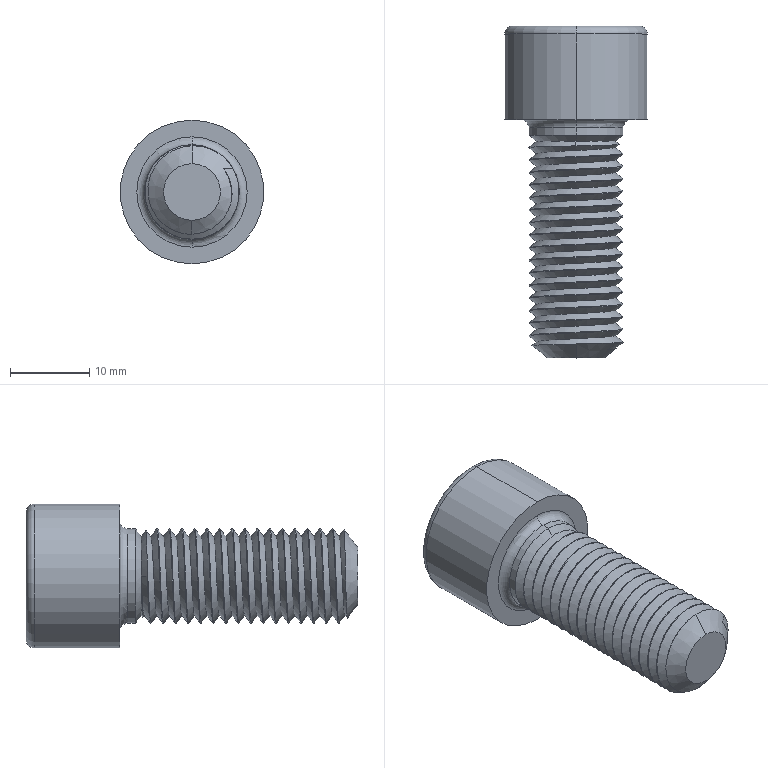Part | STEP file | Parafuso M12 - 30mm | 1 solid | 63 faces | box 18.1 x 41.8 x 18.1 mm | volume 5454 mm3 | cylinder 36 | plane 10 | cone 9 | torus 6 | spline 2 | commonest cylinder face diameters 11.9 x34 18.1 x2